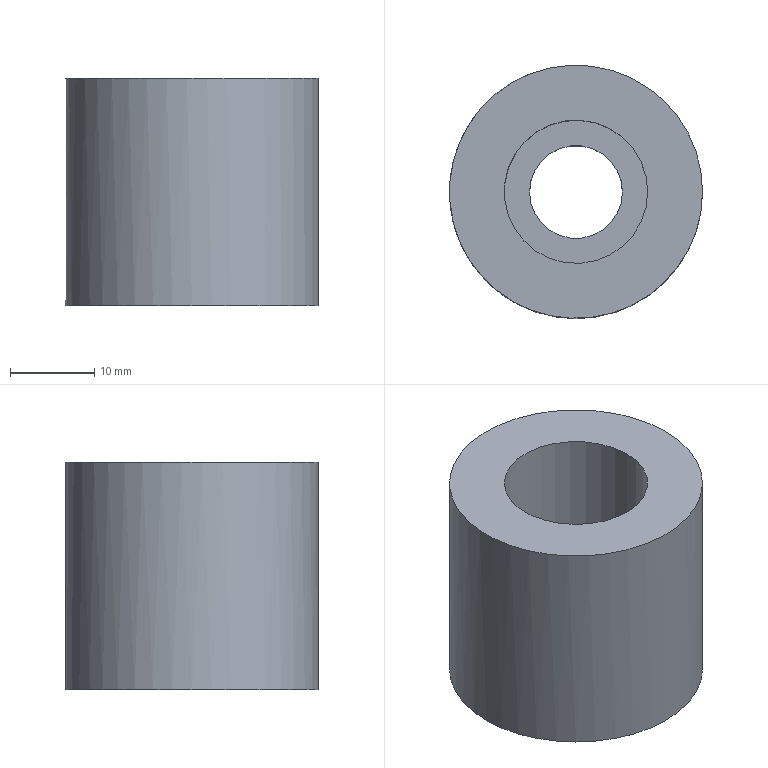Part | STEP file | 1 solid | 6 faces | box 30 x 30 x 27 mm | volume 14276 mm3 | plane 3 | cylinder 3 | commonest cylinder face diameters 11 x1 17 x1 30 x1
STEP:
#1=CARTESIAN_POINT('',(-284.,-147.5,25.));
#2=VERTEX_POINT('',#1);
#3=CARTESIAN_POINT('',(-299.,-147.5,25.));
#4=DIRECTION('',(0.,0.,-1.));
#5=DIRECTION('',(1.,0.,0.));
#6=AXIS2_PLACEMENT_3D('',#3,#4,#5);
#7=CIRCLE('',#6,15.);
#8=EDGE_CURVE('',#2,#2,#7,.T.);
#9=ORIENTED_EDGE('',*,*,#8,.F.);
#10=EDGE_LOOP('',(#9));
#11=FACE_BOUND('',#10,.T.);
#12=CARTESIAN_POINT('',(-290.5,-147.5,25.));
#13=VERTEX_POINT('',#12);
#14=CARTESIAN_POINT('',(-299.,-147.5,25.));
#15=DIRECTION('',(0.,0.,-1.));
#16=DIRECTION('',(1.,0.,0.));
#17=AXIS2_PLACEMENT_3D('',#14,#15,#16);
#18=CIRCLE('',#17,8.5);
#19=EDGE_CURVE('',#13,#13,#18,.T.);
#20=ORIENTED_EDGE('',*,*,#19,.T.);
#21=EDGE_LOOP('',(#20));
#22=FACE_BOUND('',#21,.T.);
#23=CARTESIAN_POINT('',(-299.,-147.5,25.));
#24=DIRECTION('',(0.,0.,1.));
#25=DIRECTION('',(1.,0.,0.));
#26=AXIS2_PLACEMENT_3D('',#23,#24,#25);
#27=PLANE('',#26);
#28=ADVANCED_FACE('',(#11,#22),#27,.T.);
#29=CARTESIAN_POINT('',(-314.,-147.5,-2.));
#30=VERTEX_POINT('',#29);
#31=CARTESIAN_POINT('',(-299.,-147.5,-2.));
#32=DIRECTION('',(0.,0.,1.));
#33=DIRECTION('',(-1.,0.,0.));
#34=AXIS2_PLACEMENT_3D('',#31,#32,#33);
#35=CIRCLE('',#34,15.);
#36=EDGE_CURVE('',#30,#30,#35,.T.);
#37=ORIENTED_EDGE('',*,*,#36,.F.);
#38=EDGE_LOOP('',(#37));
#39=FACE_BOUND('',#38,.T.);
#40=CARTESIAN_POINT('',(-293.5,-147.5,-2.));
#41=VERTEX_POINT('',#40);
#42=CARTESIAN_POINT('',(-299.,-147.5,-2.));
#43=DIRECTION('',(0.,0.,1.));
#44=DIRECTION('',(1.,0.,0.));
#45=AXIS2_PLACEMENT_3D('',#42,#43,#44);
#46=CIRCLE('',#45,5.5);
#47=EDGE_CURVE('',#41,#41,#46,.T.);
#48=ORIENTED_EDGE('',*,*,#47,.T.);
#49=EDGE_LOOP('',(#48));
#50=FACE_BOUND('',#49,.T.);
#51=CARTESIAN_POINT('',(-299.,-147.5,-2.));
#52=DIRECTION('',(0.,0.,-1.));
#53=DIRECTION('',(-1.,0.,0.));
#54=AXIS2_PLACEMENT_3D('',#51,#52,#53);
#55=PLANE('',#54);
#56=ADVANCED_FACE('',(#39,#50),#55,.T.);
#57=ORIENTED_EDGE('',*,*,#8,.T.);
#58=EDGE_LOOP('',(#57));
#59=FACE_BOUND('',#58,.T.);
#60=ORIENTED_EDGE('',*,*,#36,.T.);
#61=EDGE_LOOP('',(#60));
#62=FACE_BOUND('',#61,.T.);
#63=CARTESIAN_POINT('',(-299.,-147.5,-2.));
#64=DIRECTION('',(0.,0.,1.));
#65=DIRECTION('',(1.,0.,0.));
#66=AXIS2_PLACEMENT_3D('',#63,#64,#65);
#67=CYLINDRICAL_SURFACE('',#66,15.);
#68=ADVANCED_FACE('',(#59,#62),#67,.T.);
#69=CARTESIAN_POINT('',(-304.5,-147.5,8.));
#70=VERTEX_POINT('',#69);
#71=CARTESIAN_POINT('',(-299.,-147.5,8.));
#72=DIRECTION('',(0.,0.,-1.));
#73=DIRECTION('',(-1.,0.,0.));
#74=AXIS2_PLACEMENT_3D('',#71,#72,#73);
#75=CIRCLE('',#74,5.5);
#76=EDGE_CURVE('',#70,#70,#75,.T.);
#77=ORIENTED_EDGE('',*,*,#76,.F.);
#78=EDGE_LOOP('',(#77));
#79=FACE_BOUND('',#78,.T.);
#80=ORIENTED_EDGE('',*,*,#47,.F.);
#81=EDGE_LOOP('',(#80));
#82=FACE_BOUND('',#81,.T.);
#83=CARTESIAN_POINT('',(-299.,-147.5,-2.));
#84=DIRECTION('',(0.,0.,1.));
#85=DIRECTION('',(1.,0.,0.));
#86=AXIS2_PLACEMENT_3D('',#83,#84,#85);
#87=CYLINDRICAL_SURFACE('',#86,5.5);
#88=ADVANCED_FACE('',(#79,#82),#87,.F.);
#89=ORIENTED_EDGE('',*,*,#76,.T.);
#90=EDGE_LOOP('',(#89));
#91=FACE_BOUND('',#90,.T.);
#92=CARTESIAN_POINT('',(-290.5,-147.5,8.));
#93=VERTEX_POINT('',#92);
#94=CARTESIAN_POINT('',(-299.,-147.5,8.));
#95=DIRECTION('',(0.,0.,-1.));
#96=DIRECTION('',(1.,0.,0.));
#97=AXIS2_PLACEMENT_3D('',#94,#95,#96);
#98=CIRCLE('',#97,8.5);
#99=EDGE_CURVE('',#93,#93,#98,.T.);
#100=ORIENTED_EDGE('',*,*,#99,.F.);
#101=EDGE_LOOP('',(#100));
#102=FACE_BOUND('',#101,.T.);
#103=CARTESIAN_POINT('',(-299.,-147.5,8.));
#104=DIRECTION('',(0.,0.,-1.));
#105=DIRECTION('',(-1.,0.,0.));
#106=AXIS2_PLACEMENT_3D('',#103,#104,#105);
#107=PLANE('',#106);
#108=ADVANCED_FACE('',(#91,#102),#107,.F.);
#109=ORIENTED_EDGE('',*,*,#19,.F.);
#110=EDGE_LOOP('',(#109));
#111=FACE_BOUND('',#110,.T.);
#112=ORIENTED_EDGE('',*,*,#99,.T.);
#113=EDGE_LOOP('',(#112));
#114=FACE_BOUND('',#113,.T.);
#115=CARTESIAN_POINT('',(-299.,-147.5,8.));
#116=DIRECTION('',(0.,0.,1.));
#117=DIRECTION('',(1.,0.,0.));
#118=AXIS2_PLACEMENT_3D('',#115,#116,#117);
#119=CYLINDRICAL_SURFACE('',#118,8.5);
#120=ADVANCED_FACE('',(#111,#114),#119,.F.);
#121=CLOSED_SHELL('',(#28,#56,#68,#88,#108,#120));
#122=MANIFOLD_SOLID_BREP('',#121);
#123=(LENGTH_UNIT()NAMED_UNIT(*)SI_UNIT(.MILLI.,.METRE.));
#124=UNCERTAINTY_MEASURE_WITH_UNIT(LENGTH_MEASURE(0.00002),#123,'','');
#125=(NAMED_UNIT(*)PLANE_ANGLE_UNIT()SI_UNIT($,.RADIAN.));
#126=PLANE_ANGLE_MEASURE_WITH_UNIT(PLANE_ANGLE_MEASURE(0.01745),#125);
#127=DIMENSIONAL_EXPONENTS(0.,0.,0.,0.,0.,0.,0.);
#128=(CONVERSION_BASED_UNIT('DEGREE',#126)NAMED_UNIT(#127)PLANE_ANGLE_UNIT());
#129=(NAMED_UNIT(*)SI_UNIT($,.STERADIAN.)SOLID_ANGLE_UNIT());
#130=(GEOMETRIC_REPRESENTATION_CONTEXT(3)GLOBAL_UNCERTAINTY_ASSIGNED_CONTEXT((#124))GLOBAL_UNIT_ASSIGNED_CONTEXT((#123,#128,#129))REPRESENTATION_CONTEXT('',''));
#131=ADVANCED_BREP_SHAPE_REPRESENTATION('',(#122),#130);